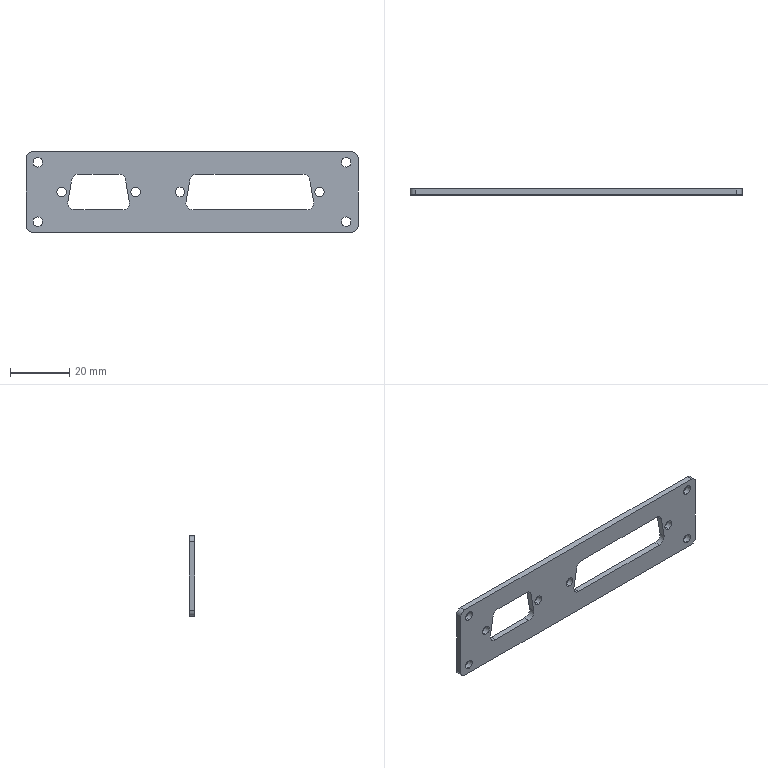Part | SolidWorks | features Cut 1, Extrusion 1, Fillet 1, ICE 1 | 1 solid | 42 faces | box 112 x 2 x 27 mm | volume 4446 mm3 | cylinder 28 | plane 14 | commonest cylinder face diameters 3.2 x16 4.8 x8 4 x4
STEP:
#1=CARTESIAN_POINT('',(43.02,0.,-1.6));
#2=VERTEX_POINT('',#1);
#3=CARTESIAN_POINT('',(43.02,0.,1.6));
#4=VERTEX_POINT('',#3);
#5=CARTESIAN_POINT('',(43.02,0.,0.));
#6=DIRECTION('',(0.,1.,0.));
#7=DIRECTION('',(0.,0.,1.));
#8=AXIS2_PLACEMENT_3D('',#5,#6,#7);
#9=CIRCLE('',#8,1.6);
#10=EDGE_CURVE('',#2,#4,#9,.T.);
#11=ORIENTED_EDGE('',*,*,#10,.F.);
#12=CARTESIAN_POINT('',(43.02,2.,-1.6));
#13=VERTEX_POINT('',#12);
#14=CARTESIAN_POINT('',(43.02,0.,-1.6));
#15=DIRECTION('',(0.,1.,0.));
#16=VECTOR('',#15,1000.);
#17=LINE('',#14,#16);
#18=EDGE_CURVE('',#2,#13,#17,.T.);
#19=ORIENTED_EDGE('',*,*,#18,.T.);
#20=CARTESIAN_POINT('',(43.02,2.,1.6));
#21=VERTEX_POINT('',#20);
#22=CARTESIAN_POINT('',(43.02,2.,0.));
#23=DIRECTION('',(0.,1.,0.));
#24=DIRECTION('',(0.,0.,1.));
#25=AXIS2_PLACEMENT_3D('',#22,#23,#24);
#26=CIRCLE('',#25,1.6);
#27=EDGE_CURVE('',#13,#21,#26,.T.);
#28=ORIENTED_EDGE('',*,*,#27,.T.);
#29=CARTESIAN_POINT('',(43.02,0.,1.6));
#30=DIRECTION('',(0.,1.,0.));
#31=VECTOR('',#30,1000.);
#32=LINE('',#29,#31);
#33=EDGE_CURVE('',#4,#21,#32,.T.);
#34=ORIENTED_EDGE('',*,*,#33,.F.);
#35=EDGE_LOOP('',(#11,#19,#28,#34));
#36=FACE_OUTER_BOUND('',#35,.T.);
#37=CARTESIAN_POINT('',(43.02,0.,0.));
#38=DIRECTION('',(0.,1.,0.));
#39=DIRECTION('',(0.,0.,1.));
#40=AXIS2_PLACEMENT_3D('',#37,#38,#39);
#41=CYLINDRICAL_SURFACE('',#40,1.6);
#42=ADVANCED_FACE('',(#36),#41,.F.);
#43=CARTESIAN_POINT('',(-4.02,0.,-1.6));
#44=VERTEX_POINT('',#43);
#45=CARTESIAN_POINT('',(-4.02,0.,1.6));
#46=VERTEX_POINT('',#45);
#47=CARTESIAN_POINT('',(-4.02,0.,0.));
#48=DIRECTION('',(0.,1.,0.));
#49=DIRECTION('',(0.,0.,1.));
#50=AXIS2_PLACEMENT_3D('',#47,#48,#49);
#51=CIRCLE('',#50,1.6);
#52=EDGE_CURVE('',#44,#46,#51,.T.);
#53=ORIENTED_EDGE('',*,*,#52,.F.);
#54=CARTESIAN_POINT('',(-4.02,2.,-1.6));
#55=VERTEX_POINT('',#54);
#56=CARTESIAN_POINT('',(-4.02,0.,-1.6));
#57=DIRECTION('',(0.,1.,0.));
#58=VECTOR('',#57,1000.);
#59=LINE('',#56,#58);
#60=EDGE_CURVE('',#44,#55,#59,.T.);
#61=ORIENTED_EDGE('',*,*,#60,.T.);
#62=CARTESIAN_POINT('',(-4.02,2.,1.6));
#63=VERTEX_POINT('',#62);
#64=CARTESIAN_POINT('',(-4.02,2.,0.));
#65=DIRECTION('',(0.,1.,0.));
#66=DIRECTION('',(0.,0.,1.));
#67=AXIS2_PLACEMENT_3D('',#64,#65,#66);
#68=CIRCLE('',#67,1.6);
#69=EDGE_CURVE('',#55,#63,#68,.T.);
#70=ORIENTED_EDGE('',*,*,#69,.T.);
#71=CARTESIAN_POINT('',(-4.02,0.,1.6));
#72=DIRECTION('',(0.,1.,0.));
#73=VECTOR('',#72,1000.);
#74=LINE('',#71,#73);
#75=EDGE_CURVE('',#46,#63,#74,.T.);
#76=ORIENTED_EDGE('',*,*,#75,.F.);
#77=EDGE_LOOP('',(#53,#61,#70,#76));
#78=FACE_OUTER_BOUND('',#77,.T.);
#79=CARTESIAN_POINT('',(-4.02,0.,0.));
#80=DIRECTION('',(0.,1.,0.));
#81=DIRECTION('',(0.,0.,1.));
#82=AXIS2_PLACEMENT_3D('',#79,#80,#81);
#83=CYLINDRICAL_SURFACE('',#82,1.6);
#84=ADVANCED_FACE('',(#78),#83,.F.);
#85=CARTESIAN_POINT('',(-19.005,0.,-1.6));
#86=VERTEX_POINT('',#85);
#87=CARTESIAN_POINT('',(-19.005,0.,1.6));
#88=VERTEX_POINT('',#87);
#89=CARTESIAN_POINT('',(-19.005,0.,0.));
#90=DIRECTION('',(0.,1.,0.));
#91=DIRECTION('',(0.,0.,1.));
#92=AXIS2_PLACEMENT_3D('',#89,#90,#91);
#93=CIRCLE('',#92,1.6);
#94=EDGE_CURVE('',#86,#88,#93,.T.);
#95=ORIENTED_EDGE('',*,*,#94,.F.);
#96=CARTESIAN_POINT('',(-19.005,2.,-1.6));
#97=VERTEX_POINT('',#96);
#98=CARTESIAN_POINT('',(-19.005,0.,-1.6));
#99=DIRECTION('',(0.,1.,0.));
#100=VECTOR('',#99,1000.);
#101=LINE('',#98,#100);
#102=EDGE_CURVE('',#86,#97,#101,.T.);
#103=ORIENTED_EDGE('',*,*,#102,.T.);
#104=CARTESIAN_POINT('',(-19.005,2.,1.6));
#105=VERTEX_POINT('',#104);
#106=CARTESIAN_POINT('',(-19.005,2.,0.));
#107=DIRECTION('',(0.,1.,0.));
#108=DIRECTION('',(0.,0.,1.));
#109=AXIS2_PLACEMENT_3D('',#106,#107,#108);
#110=CIRCLE('',#109,1.6);
#111=EDGE_CURVE('',#97,#105,#110,.T.);
#112=ORIENTED_EDGE('',*,*,#111,.T.);
#113=CARTESIAN_POINT('',(-19.005,0.,1.6));
#114=DIRECTION('',(0.,1.,0.));
#115=VECTOR('',#114,1000.);
#116=LINE('',#113,#115);
#117=EDGE_CURVE('',#88,#105,#116,.T.);
#118=ORIENTED_EDGE('',*,*,#117,.F.);
#119=EDGE_LOOP('',(#95,#103,#112,#118));
#120=FACE_OUTER_BOUND('',#119,.T.);
#121=CARTESIAN_POINT('',(-19.005,0.,0.));
#122=DIRECTION('',(0.,1.,0.));
#123=DIRECTION('',(0.,0.,1.));
#124=AXIS2_PLACEMENT_3D('',#121,#122,#123);
#125=CYLINDRICAL_SURFACE('',#124,1.6);
#126=ADVANCED_FACE('',(#120),#125,.F.);
#127=CARTESIAN_POINT('',(-43.995,0.,-1.6));
#128=VERTEX_POINT('',#127);
#129=CARTESIAN_POINT('',(-43.995,0.,1.6));
#130=VERTEX_POINT('',#129);
#131=CARTESIAN_POINT('',(-43.995,0.,0.));
#132=DIRECTION('',(0.,1.,0.));
#133=DIRECTION('',(0.,0.,1.));
#134=AXIS2_PLACEMENT_3D('',#131,#132,#133);
#135=CIRCLE('',#134,1.6);
#136=EDGE_CURVE('',#128,#130,#135,.T.);
#137=ORIENTED_EDGE('',*,*,#136,.F.);
#138=CARTESIAN_POINT('',(-43.995,2.,-1.6));
#139=VERTEX_POINT('',#138);
#140=CARTESIAN_POINT('',(-43.995,0.,-1.6));
#141=DIRECTION('',(0.,1.,0.));
#142=VECTOR('',#141,1000.);
#143=LINE('',#140,#142);
#144=EDGE_CURVE('',#128,#139,#143,.T.);
#145=ORIENTED_EDGE('',*,*,#144,.T.);
#146=CARTESIAN_POINT('',(-43.995,2.,1.6));
#147=VERTEX_POINT('',#146);
#148=CARTESIAN_POINT('',(-43.995,2.,0.));
#149=DIRECTION('',(0.,1.,0.));
#150=DIRECTION('',(0.,0.,1.));
#151=AXIS2_PLACEMENT_3D('',#148,#149,#150);
#152=CIRCLE('',#151,1.6);
#153=EDGE_CURVE('',#139,#147,#152,.T.);
#154=ORIENTED_EDGE('',*,*,#153,.T.);
#155=CARTESIAN_POINT('',(-43.995,0.,1.6));
#156=DIRECTION('',(0.,1.,0.));
#157=VECTOR('',#156,1000.);
#158=LINE('',#155,#157);
#159=EDGE_CURVE('',#130,#147,#158,.T.);
#160=ORIENTED_EDGE('',*,*,#159,.F.);
#161=EDGE_LOOP('',(#137,#145,#154,#160));
#162=FACE_OUTER_BOUND('',#161,.T.);
#163=CARTESIAN_POINT('',(-43.995,0.,0.));
#164=DIRECTION('',(0.,1.,0.));
#165=DIRECTION('',(0.,0.,1.));
#166=AXIS2_PLACEMENT_3D('',#163,#164,#165);
#167=CYLINDRICAL_SURFACE('',#166,1.6);
#168=ADVANCED_FACE('',(#162),#167,.F.);
#169=CARTESIAN_POINT('',(-52.,0.,8.4));
#170=VERTEX_POINT('',#169);
#171=CARTESIAN_POINT('',(-52.,0.,11.6));
#172=VERTEX_POINT('',#171);
#173=CARTESIAN_POINT('',(-52.,0.,10.));
#174=DIRECTION('',(0.,1.,0.));
#175=DIRECTION('',(0.,0.,1.));
#176=AXIS2_PLACEMENT_3D('',#173,#174,#175);
#177=CIRCLE('',#176,1.6);
#178=EDGE_CURVE('',#170,#172,#177,.T.);
#179=ORIENTED_EDGE('',*,*,#178,.F.);
#180=CARTESIAN_POINT('',(-52.,2.,8.4));
#181=VERTEX_POINT('',#180);
#182=CARTESIAN_POINT('',(-52.,0.,8.4));
#183=DIRECTION('',(0.,1.,0.));
#184=VECTOR('',#183,1000.);
#185=LINE('',#182,#184);
#186=EDGE_CURVE('',#170,#181,#185,.T.);
#187=ORIENTED_EDGE('',*,*,#186,.T.);
#188=CARTESIAN_POINT('',(-52.,2.,11.6));
#189=VERTEX_POINT('',#188);
#190=CARTESIAN_POINT('',(-52.,2.,10.));
#191=DIRECTION('',(0.,1.,0.));
#192=DIRECTION('',(0.,0.,1.));
#193=AXIS2_PLACEMENT_3D('',#190,#191,#192);
#194=CIRCLE('',#193,1.6);
#195=EDGE_CURVE('',#181,#189,#194,.T.);
#196=ORIENTED_EDGE('',*,*,#195,.T.);
#197=CARTESIAN_POINT('',(-52.,0.,11.6));
#198=DIRECTION('',(0.,1.,0.));
#199=VECTOR('',#198,1000.);
#200=LINE('',#197,#199);
#201=EDGE_CURVE('',#172,#189,#200,.T.);
#202=ORIENTED_EDGE('',*,*,#201,.F.);
#203=EDGE_LOOP('',(#179,#187,#196,#202));
#204=FACE_OUTER_BOUND('',#203,.T.);
#205=CARTESIAN_POINT('',(-52.,0.,10.));
#206=DIRECTION('',(0.,1.,0.));
#207=DIRECTION('',(0.,0.,1.));
#208=AXIS2_PLACEMENT_3D('',#205,#206,#207);
#209=CYLINDRICAL_SURFACE('',#208,1.6);
#210=ADVANCED_FACE('',(#204),#209,.F.);
#211=CARTESIAN_POINT('',(52.,0.,8.4));
#212=VERTEX_POINT('',#211);
#213=CARTESIAN_POINT('',(52.,0.,11.6));
#214=VERTEX_POINT('',#213);
#215=CARTESIAN_POINT('',(52.,0.,10.));
#216=DIRECTION('',(0.,1.,0.));
#217=DIRECTION('',(0.,0.,1.));
#218=AXIS2_PLACEMENT_3D('',#215,#216,#217);
#219=CIRCLE('',#218,1.6);
#220=EDGE_CURVE('',#212,#214,#219,.T.);
#221=ORIENTED_EDGE('',*,*,#220,.F.);
#222=CARTESIAN_POINT('',(52.,2.,8.4));
#223=VERTEX_POINT('',#222);
#224=CARTESIAN_POINT('',(52.,0.,8.4));
#225=DIRECTION('',(0.,1.,0.));
#226=VECTOR('',#225,1000.);
#227=LINE('',#224,#226);
#228=EDGE_CURVE('',#212,#223,#227,.T.);
#229=ORIENTED_EDGE('',*,*,#228,.T.);
#230=CARTESIAN_POINT('',(52.,2.,11.6));
#231=VERTEX_POINT('',#230);
#232=CARTESIAN_POINT('',(52.,2.,10.));
#233=DIRECTION('',(0.,1.,0.));
#234=DIRECTION('',(0.,0.,1.));
#235=AXIS2_PLACEMENT_3D('',#232,#233,#234);
#236=CIRCLE('',#235,1.6);
#237=EDGE_CURVE('',#223,#231,#236,.T.);
#238=ORIENTED_EDGE('',*,*,#237,.T.);
#239=CARTESIAN_POINT('',(52.,0.,11.6));
#240=DIRECTION('',(0.,1.,0.));
#241=VECTOR('',#240,1000.);
#242=LINE('',#239,#241);
#243=EDGE_CURVE('',#214,#231,#242,.T.);
#244=ORIENTED_EDGE('',*,*,#243,.F.);
#245=EDGE_LOOP('',(#221,#229,#238,#244));
#246=FACE_OUTER_BOUND('',#245,.T.);
#247=CARTESIAN_POINT('',(52.,0.,10.));
#248=DIRECTION('',(0.,1.,0.));
#249=DIRECTION('',(0.,0.,1.));
#250=AXIS2_PLACEMENT_3D('',#247,#248,#249);
#251=CYLINDRICAL_SURFACE('',#250,1.6);
#252=ADVANCED_FACE('',(#246),#251,.F.);
#253=CARTESIAN_POINT('',(52.,0.,-11.6));
#254=VERTEX_POINT('',#253);
#255=CARTESIAN_POINT('',(52.,0.,-8.4));
#256=VERTEX_POINT('',#255);
#257=CARTESIAN_POINT('',(52.,0.,-10.));
#258=DIRECTION('',(0.,1.,0.));
#259=DIRECTION('',(0.,0.,1.));
#260=AXIS2_PLACEMENT_3D('',#257,#258,#259);
#261=CIRCLE('',#260,1.6);
#262=EDGE_CURVE('',#254,#256,#261,.T.);
#263=ORIENTED_EDGE('',*,*,#262,.F.);
#264=CARTESIAN_POINT('',(52.,2.,-11.6));
#265=VERTEX_POINT('',#264);
#266=CARTESIAN_POINT('',(52.,0.,-11.6));
#267=DIRECTION('',(0.,1.,0.));
#268=VECTOR('',#267,1000.);
#269=LINE('',#266,#268);
#270=EDGE_CURVE('',#254,#265,#269,.T.);
#271=ORIENTED_EDGE('',*,*,#270,.T.);
#272=CARTESIAN_POINT('',(52.,2.,-8.4));
#273=VERTEX_POINT('',#272);
#274=CARTESIAN_POINT('',(52.,2.,-10.));
#275=DIRECTION('',(0.,1.,0.));
#276=DIRECTION('',(0.,0.,1.));
#277=AXIS2_PLACEMENT_3D('',#274,#275,#276);
#278=CIRCLE('',#277,1.6);
#279=EDGE_CURVE('',#265,#273,#278,.T.);
#280=ORIENTED_EDGE('',*,*,#279,.T.);
#281=CARTESIAN_POINT('',(52.,0.,-8.4));
#282=DIRECTION('',(0.,1.,0.));
#283=VECTOR('',#282,1000.);
#284=LINE('',#281,#283);
#285=EDGE_CURVE('',#256,#273,#284,.T.);
#286=ORIENTED_EDGE('',*,*,#285,.F.);
#287=EDGE_LOOP('',(#263,#271,#280,#286));
#288=FACE_OUTER_BOUND('',#287,.T.);
#289=CARTESIAN_POINT('',(52.,0.,-10.));
#290=DIRECTION('',(0.,1.,0.));
#291=DIRECTION('',(0.,0.,1.));
#292=AXIS2_PLACEMENT_3D('',#289,#290,#291);
#293=CYLINDRICAL_SURFACE('',#292,1.6);
#294=ADVANCED_FACE('',(#288),#293,.F.);
#295=CARTESIAN_POINT('',(-52.,0.,-11.6));
#296=VERTEX_POINT('',#295);
#297=CARTESIAN_POINT('',(-52.,0.,-8.4));
#298=VERTEX_POINT('',#297);
#299=CARTESIAN_POINT('',(-52.,0.,-10.));
#300=DIRECTION('',(0.,1.,0.));
#301=DIRECTION('',(0.,0.,1.));
#302=AXIS2_PLACEMENT_3D('',#299,#300,#301);
#303=CIRCLE('',#302,1.6);
#304=EDGE_CURVE('',#296,#298,#303,.T.);
#305=ORIENTED_EDGE('',*,*,#304,.F.);
#306=CARTESIAN_POINT('',(-52.,2.,-11.6));
#307=VERTEX_POINT('',#306);
#308=CARTESIAN_POINT('',(-52.,0.,-11.6));
#309=DIRECTION('',(0.,1.,0.));
#310=VECTOR('',#309,1000.);
#311=LINE('',#308,#310);
#312=EDGE_CURVE('',#296,#307,#311,.T.);
#313=ORIENTED_EDGE('',*,*,#312,.T.);
#314=CARTESIAN_POINT('',(-52.,2.,-8.4));
#315=VERTEX_POINT('',#314);
#316=CARTESIAN_POINT('',(-52.,2.,-10.));
#317=DIRECTION('',(0.,1.,0.));
#318=DIRECTION('',(0.,0.,1.));
#319=AXIS2_PLACEMENT_3D('',#316,#317,#318);
#320=CIRCLE('',#319,1.6);
#321=EDGE_CURVE('',#307,#315,#320,.T.);
#322=ORIENTED_EDGE('',*,*,#321,.T.);
#323=CARTESIAN_POINT('',(-52.,0.,-8.4));
#324=DIRECTION('',(0.,1.,0.));
#325=VECTOR('',#324,1000.);
#326=LINE('',#323,#325);
#327=EDGE_CURVE('',#298,#315,#326,.T.);
#328=ORIENTED_EDGE('',*,*,#327,.F.);
#329=EDGE_LOOP('',(#305,#313,#322,#328));
#330=FACE_OUTER_BOUND('',#329,.T.);
#331=CARTESIAN_POINT('',(-52.,0.,-10.));
#332=DIRECTION('',(0.,1.,0.));
#333=DIRECTION('',(0.,0.,1.));
#334=AXIS2_PLACEMENT_3D('',#331,#332,#333);
#335=CYLINDRICAL_SURFACE('',#334,1.6);
#336=ADVANCED_FACE('',(#330),#335,.F.);
#337=CARTESIAN_POINT('',(43.02,2.,0.));
#338=DIRECTION('',(0.,1.,0.));
#339=DIRECTION('',(0.,0.,1.));
#340=AXIS2_PLACEMENT_3D('',#337,#338,#339);
#341=CIRCLE('',#340,1.6);
#342=EDGE_CURVE('',#21,#13,#341,.T.);
#343=ORIENTED_EDGE('',*,*,#342,.F.);
#344=ORIENTED_EDGE('',*,*,#27,.F.);
#345=EDGE_LOOP('',(#343,#344));
#346=FACE_BOUND('',#345,.T.);
#347=CARTESIAN_POINT('',(-39.5,2.,-6.05));
#348=VERTEX_POINT('',#347);
#349=CARTESIAN_POINT('',(-23.5,2.,-6.05));
#350=VERTEX_POINT('',#349);
#351=CARTESIAN_POINT('',(0.,2.,-6.05));
#352=DIRECTION('',(1.,0.,0.));
#353=VECTOR('',#352,1000.);
#354=LINE('',#351,#353);
#355=EDGE_CURVE('',#348,#350,#354,.T.);
#356=ORIENTED_EDGE('',*,*,#355,.T.);
#357=CARTESIAN_POINT('',(-21.136,2.,-3.233));
#358=VERTEX_POINT('',#357);
#359=CARTESIAN_POINT('',(-23.5,2.,-3.65));
#360=DIRECTION('',(0.,-1.,0.));
#361=DIRECTION('',(0.,0.,1.));
#362=AXIS2_PLACEMENT_3D('',#359,#360,#361);
#363=CIRCLE('',#362,2.4);
#364=EDGE_CURVE('',#350,#358,#363,.T.);
#365=ORIENTED_EDGE('',*,*,#364,.T.);
#366=CARTESIAN_POINT('',(-22.424,2.,4.067));
#367=VERTEX_POINT('',#366);
#368=CARTESIAN_POINT('',(-21.052,2.,-3.712));
#369=DIRECTION('',(-0.1736,0.,0.9848));
#370=VECTOR('',#369,1000.);
#371=LINE('',#368,#370);
#372=EDGE_CURVE('',#358,#367,#371,.T.);
#373=ORIENTED_EDGE('',*,*,#372,.T.);
#374=CARTESIAN_POINT('',(-24.787,2.,6.05));
#375=VERTEX_POINT('',#374);
#376=CARTESIAN_POINT('',(-24.787,2.,3.65));
#377=DIRECTION('',(0.,-1.,0.));
#378=DIRECTION('',(0.,0.,1.));
#379=AXIS2_PLACEMENT_3D('',#376,#377,#378);
#380=CIRCLE('',#379,2.4);
#381=EDGE_CURVE('',#367,#375,#380,.T.);
#382=ORIENTED_EDGE('',*,*,#381,.T.);
#383=CARTESIAN_POINT('',(-38.213,2.,6.05));
#384=VERTEX_POINT('',#383);
#385=CARTESIAN_POINT('',(0.,2.,6.05));
#386=DIRECTION('',(-1.,0.,0.));
#387=VECTOR('',#386,1000.);
#388=LINE('',#385,#387);
#389=EDGE_CURVE('',#375,#384,#388,.T.);
#390=ORIENTED_EDGE('',*,*,#389,.T.);
#391=CARTESIAN_POINT('',(-40.576,2.,4.067));
#392=VERTEX_POINT('',#391);
#393=CARTESIAN_POINT('',(-38.213,2.,3.65));
#394=DIRECTION('',(0.,-1.,0.));
#395=DIRECTION('',(0.,0.,1.));
#396=AXIS2_PLACEMENT_3D('',#393,#394,#395);
#397=CIRCLE('',#396,2.4);
#398=EDGE_CURVE('',#384,#392,#397,.T.);
#399=ORIENTED_EDGE('',*,*,#398,.T.);
#400=CARTESIAN_POINT('',(-41.864,2.,-3.233));
#401=VERTEX_POINT('',#400);
#402=CARTESIAN_POINT('',(-40.048,2.,7.062));
#403=DIRECTION('',(-0.1736,0.,-0.9848));
#404=VECTOR('',#403,1000.);
#405=LINE('',#402,#404);
#406=EDGE_CURVE('',#392,#401,#405,.T.);
#407=ORIENTED_EDGE('',*,*,#406,.T.);
#408=CARTESIAN_POINT('',(-39.5,2.,-3.65));
#409=DIRECTION('',(0.,1.,0.));
#410=DIRECTION('',(0.,0.,1.));
#411=AXIS2_PLACEMENT_3D('',#408,#409,#410);
#412=CIRCLE('',#411,2.4);
#413=EDGE_CURVE('',#348,#401,#412,.T.);
#414=ORIENTED_EDGE('',*,*,#413,.F.);
#415=EDGE_LOOP('',(#356,#365,#373,#382,#390,#399,#407,#414));
#416=FACE_BOUND('',#415,.T.);
#417=CARTESIAN_POINT('',(-52.,2.,10.));
#418=DIRECTION('',(0.,1.,0.));
#419=DIRECTION('',(0.,0.,1.));
#420=AXIS2_PLACEMENT_3D('',#417,#418,#419);
#421=CIRCLE('',#420,1.6);
#422=EDGE_CURVE('',#189,#181,#421,.T.);
#423=ORIENTED_EDGE('',*,*,#422,.F.);
#424=ORIENTED_EDGE('',*,*,#195,.F.);
#425=EDGE_LOOP('',(#423,#424));
#426=FACE_BOUND('',#425,.T.);
#427=CARTESIAN_POINT('',(52.,2.,10.));
#428=DIRECTION('',(0.,1.,0.));
#429=DIRECTION('',(0.,0.,1.));
#430=AXIS2_PLACEMENT_3D('',#427,#428,#429);
#431=CIRCLE('',#430,1.6);
#432=EDGE_CURVE('',#231,#223,#431,.T.);
#433=ORIENTED_EDGE('',*,*,#432,.F.);
#434=ORIENTED_EDGE('',*,*,#237,.F.);
#435=EDGE_LOOP('',(#433,#434));
#436=FACE_BOUND('',#435,.T.);
#437=CARTESIAN_POINT('',(52.,2.,-10.));
#438=DIRECTION('',(0.,1.,0.));
#439=DIRECTION('',(0.,0.,1.));
#440=AXIS2_PLACEMENT_3D('',#437,#438,#439);
#441=CIRCLE('',#440,1.6);
#442=EDGE_CURVE('',#273,#265,#441,.T.);
#443=ORIENTED_EDGE('',*,*,#442,.F.);
#444=ORIENTED_EDGE('',*,*,#279,.F.);
#445=EDGE_LOOP('',(#443,#444));
#446=FACE_BOUND('',#445,.T.);
#447=CARTESIAN_POINT('',(-52.,2.,-10.));
#448=DIRECTION('',(0.,1.,0.));
#449=DIRECTION('',(0.,0.,1.));
#450=AXIS2_PLACEMENT_3D('',#447,#448,#449);
#451=CIRCLE('',#450,1.6);
#452=EDGE_CURVE('',#315,#307,#451,.T.);
#453=ORIENTED_EDGE('',*,*,#452,.F.);
#454=ORIENTED_EDGE('',*,*,#321,.F.);
#455=EDGE_LOOP('',(#453,#454));
#456=FACE_BOUND('',#455,.T.);
#457=CARTESIAN_POINT('',(56.,2.,11.5));
#458=VERTEX_POINT('',#457);
#459=CARTESIAN_POINT('',(56.,2.,-11.5));
#460=VERTEX_POINT('',#459);
#461=CARTESIAN_POINT('',(56.,2.,13.5));
#462=DIRECTION('',(0.,0.,-1.));
#463=VECTOR('',#462,1000.);
#464=LINE('',#461,#463);
#465=EDGE_CURVE('',#458,#460,#464,.T.);
#466=ORIENTED_EDGE('',*,*,#465,.T.);
#467=CARTESIAN_POINT('',(54.,2.,-13.5));
#468=VERTEX_POINT('',#467);
#469=CARTESIAN_POINT('',(54.,2.,-11.5));
#470=DIRECTION('',(0.,1.,0.));
#471=DIRECTION('',(0.,0.,-1.));
#472=AXIS2_PLACEMENT_3D('',#469,#470,#471);
#473=CIRCLE('',#472,2.);
#474=EDGE_CURVE('',#460,#468,#473,.T.);
#475=ORIENTED_EDGE('',*,*,#474,.T.);
#476=CARTESIAN_POINT('',(-54.,2.,-13.5));
#477=VERTEX_POINT('',#476);
#478=CARTESIAN_POINT('',(-56.,2.,-13.5));
#479=DIRECTION('',(-1.,0.,0.));
#480=VECTOR('',#479,1000.);
#481=LINE('',#478,#480);
#482=EDGE_CURVE('',#468,#477,#481,.T.);
#483=ORIENTED_EDGE('',*,*,#482,.T.);
#484=CARTESIAN_POINT('',(-56.,2.,-11.5));
#485=VERTEX_POINT('',#484);
#486=CARTESIAN_POINT('',(-54.,2.,-11.5));
#487=DIRECTION('',(0.,1.,0.));
#488=DIRECTION('',(0.,0.,-1.));
#489=AXIS2_PLACEMENT_3D('',#486,#487,#488);
#490=CIRCLE('',#489,2.);
#491=EDGE_CURVE('',#477,#485,#490,.T.);
#492=ORIENTED_EDGE('',*,*,#491,.T.);
#493=CARTESIAN_POINT('',(-56.,2.,11.5));
#494=VERTEX_POINT('',#493);
#495=CARTESIAN_POINT('',(-56.,2.,13.5));
#496=DIRECTION('',(0.,0.,1.));
#497=VECTOR('',#496,1000.);
#498=LINE('',#495,#497);
#499=EDGE_CURVE('',#485,#494,#498,.T.);
#500=ORIENTED_EDGE('',*,*,#499,.T.);
#501=CARTESIAN_POINT('',(-54.,2.,13.5));
#502=VERTEX_POINT('',#501);
#503=CARTESIAN_POINT('',(-54.,2.,11.5));
#504=DIRECTION('',(0.,1.,0.));
#505=DIRECTION('',(0.,0.,-1.));
#506=AXIS2_PLACEMENT_3D('',#503,#504,#505);
#507=CIRCLE('',#506,2.);
#508=EDGE_CURVE('',#494,#502,#507,.T.);
#509=ORIENTED_EDGE('',*,*,#508,.T.);
#510=CARTESIAN_POINT('',(54.,2.,13.5));
#511=VERTEX_POINT('',#510);
#512=CARTESIAN_POINT('',(-56.,2.,13.5));
#513=DIRECTION('',(1.,0.,0.));
#514=VECTOR('',#513,1000.);
#515=LINE('',#512,#514);
#516=EDGE_CURVE('',#502,#511,#515,.T.);
#517=ORIENTED_EDGE('',*,*,#516,.T.);
#518=CARTESIAN_POINT('',(54.,2.,11.5));
#519=DIRECTION('',(0.,1.,0.));
#520=DIRECTION('',(0.,0.,-1.));
#521=AXIS2_PLACEMENT_3D('',#518,#519,#520);
#522=CIRCLE('',#521,2.);
#523=EDGE_CURVE('',#511,#458,#522,.T.);
#524=ORIENTED_EDGE('',*,*,#523,.T.);
#525=EDGE_LOOP('',(#466,#475,#483,#492,#500,#509,#517,#524));
#526=FACE_OUTER_BOUND('',#525,.T.);
#527=CARTESIAN_POINT('',(-43.995,2.,0.));
#528=DIRECTION('',(0.,1.,0.));
#529=DIRECTION('',(0.,0.,1.));
#530=AXIS2_PLACEMENT_3D('',#527,#528,#529);
#531=CIRCLE('',#530,1.6);
#532=EDGE_CURVE('',#147,#139,#531,.T.);
#533=ORIENTED_EDGE('',*,*,#532,.F.);
#534=ORIENTED_EDGE('',*,*,#153,.F.);
#535=EDGE_LOOP('',(#533,#534));
#536=FACE_BOUND('',#535,.T.);
#537=CARTESIAN_POINT('',(-19.005,2.,0.));
#538=DIRECTION('',(0.,1.,0.));
#539=DIRECTION('',(0.,0.,1.));
#540=AXIS2_PLACEMENT_3D('',#537,#538,#539);
#541=CIRCLE('',#540,1.6);
#542=EDGE_CURVE('',#105,#97,#541,.T.);
#543=ORIENTED_EDGE('',*,*,#542,.F.);
#544=ORIENTED_EDGE('',*,*,#111,.F.);
#545=EDGE_LOOP('',(#543,#544));
#546=FACE_BOUND('',#545,.T.);
#547=CARTESIAN_POINT('',(-4.02,2.,0.));
#548=DIRECTION('',(0.,1.,0.));
#549=DIRECTION('',(0.,0.,1.));
#550=AXIS2_PLACEMENT_3D('',#547,#548,#549);
#551=CIRCLE('',#550,1.6);
#552=EDGE_CURVE('',#63,#55,#551,.T.);
#553=ORIENTED_EDGE('',*,*,#552,.F.);
#554=ORIENTED_EDGE('',*,*,#69,.F.);
#555=EDGE_LOOP('',(#553,#554));
#556=FACE_BOUND('',#555,.T.);
#557=CARTESIAN_POINT('',(39.726,2.,4.067));
#558=VERTEX_POINT('',#557);
#559=CARTESIAN_POINT('',(37.363,2.,6.05));
#560=VERTEX_POINT('',#559);
#561=CARTESIAN_POINT('',(37.363,2.,3.65));
#562=DIRECTION('',(0.,-1.,0.));
#563=DIRECTION('',(0.,0.,1.));
#564=AXIS2_PLACEMENT_3D('',#561,#562,#563);
#565=CIRCLE('',#564,2.4);
#566=EDGE_CURVE('',#558,#560,#565,.T.);
#567=ORIENTED_EDGE('',*,*,#566,.T.);
#568=CARTESIAN_POINT('',(1.637,2.,6.05));
#569=VERTEX_POINT('',#568);
#570=CARTESIAN_POINT('',(0.,2.,6.05));
#571=DIRECTION('',(-1.,0.,0.));
#572=VECTOR('',#571,1000.);
#573=LINE('',#570,#572);
#574=EDGE_CURVE('',#560,#569,#573,.T.);
#575=ORIENTED_EDGE('',*,*,#574,.T.);
#576=CARTESIAN_POINT('',(-0.7264,2.,4.067));
#577=VERTEX_POINT('',#576);
#578=CARTESIAN_POINT('',(1.637,2.,3.65));
#579=DIRECTION('',(0.,-1.,0.));
#580=DIRECTION('',(0.,0.,1.));
#581=AXIS2_PLACEMENT_3D('',#578,#579,#580);
#582=CIRCLE('',#581,2.4);
#583=EDGE_CURVE('',#569,#577,#582,.T.);
#584=ORIENTED_EDGE('',*,*,#583,.T.);
#585=CARTESIAN_POINT('',(-2.014,2.,-3.233));
#586=VERTEX_POINT('',#585);
#587=CARTESIAN_POINT('',(-1.4,2.,0.2468));
#588=DIRECTION('',(-0.1736,0.,-0.9848));
#589=VECTOR('',#588,1000.);
#590=LINE('',#587,#589);
#591=EDGE_CURVE('',#577,#586,#590,.T.);
#592=ORIENTED_EDGE('',*,*,#591,.T.);
#593=CARTESIAN_POINT('',(0.35,2.,-6.05));
#594=VERTEX_POINT('',#593);
#595=CARTESIAN_POINT('',(0.35,2.,-3.65));
#596=DIRECTION('',(0.,1.,0.));
#597=DIRECTION('',(0.,0.,1.));
#598=AXIS2_PLACEMENT_3D('',#595,#596,#597);
#599=CIRCLE('',#598,2.4);
#600=EDGE_CURVE('',#594,#586,#599,.T.);
#601=ORIENTED_EDGE('',*,*,#600,.F.);
#602=CARTESIAN_POINT('',(38.65,2.,-6.05));
#603=VERTEX_POINT('',#602);
#604=CARTESIAN_POINT('',(0.,2.,-6.05));
#605=DIRECTION('',(1.,0.,0.));
#606=VECTOR('',#605,1000.);
#607=LINE('',#604,#606);
#608=EDGE_CURVE('',#594,#603,#607,.T.);
#609=ORIENTED_EDGE('',*,*,#608,.T.);
#610=CARTESIAN_POINT('',(41.014,2.,-3.233));
#611=VERTEX_POINT('',#610);
#612=CARTESIAN_POINT('',(38.65,2.,-3.65));
#613=DIRECTION('',(0.,-1.,0.));
#614=DIRECTION('',(0.,0.,1.));
#615=AXIS2_PLACEMENT_3D('',#612,#613,#614);
#616=CIRCLE('',#615,2.4);
#617=EDGE_CURVE('',#603,#611,#616,.T.);
#618=ORIENTED_EDGE('',*,*,#617,.T.);
#619=CARTESIAN_POINT('',(39.224,2.,6.916));
#620=DIRECTION('',(-0.1736,0.,0.9848));
#621=VECTOR('',#620,1000.);
#622=LINE('',#619,#621);
#623=EDGE_CURVE('',#611,#558,#622,.T.);
#624=ORIENTED_EDGE('',*,*,#623,.T.);
#625=EDGE_LOOP('',(#567,#575,#584,#592,#601,#609,#618,#624));
#626=FACE_BOUND('',#625,.T.);
#627=CARTESIAN_POINT('',(0.,2.,0.));
#628=DIRECTION('',(0.,-1.,0.));
#629=DIRECTION('',(0.,0.,-1.));
#630=AXIS2_PLACEMENT_3D('',#627,#628,#629);
#631=PLANE('',#630);
#632=ADVANCED_FACE('',(#346,#416,#426,#436,#446,#456,#526,#536,#546,#556,#626),#631,.F.);
#633=CARTESIAN_POINT('',(43.02,0.,0.));
#634=DIRECTION('',(0.,1.,0.));
#635=DIRECTION('',(0.,0.,1.));
#636=AXIS2_PLACEMENT_3D('',#633,#634,#635);
#637=CIRCLE('',#636,1.6);
#638=EDGE_CURVE('',#4,#2,#637,.T.);
#639=ORIENTED_EDGE('',*,*,#638,.T.);
#640=ORIENTED_EDGE('',*,*,#10,.T.);
#641=EDGE_LOOP('',(#639,#640));
#642=FACE_BOUND('',#641,.T.);
#643=CARTESIAN_POINT('',(-4.02,0.,0.));
#644=DIRECTION('',(0.,1.,0.));
#645=DIRECTION('',(0.,0.,1.));
#646=AXIS2_PLACEMENT_3D('',#643,#644,#645);
#647=CIRCLE('',#646,1.6);
#648=EDGE_CURVE('',#46,#44,#647,.T.);
#649=ORIENTED_EDGE('',*,*,#648,.T.);
#650=ORIENTED_EDGE('',*,*,#52,.T.);
#651=EDGE_LOOP('',(#649,#650));
#652=FACE_BOUND('',#651,.T.);
#653=CARTESIAN_POINT('',(-19.005,0.,0.));
#654=DIRECTION('',(0.,1.,0.));
#655=DIRECTION('',(0.,0.,1.));
#656=AXIS2_PLACEMENT_3D('',#653,#654,#655);
#657=CIRCLE('',#656,1.6);
#658=EDGE_CURVE('',#88,#86,#657,.T.);
#659=ORIENTED_EDGE('',*,*,#658,.T.);
#660=ORIENTED_EDGE('',*,*,#94,.T.);
#661=EDGE_LOOP('',(#659,#660));
#662=FACE_BOUND('',#661,.T.);
#663=CARTESIAN_POINT('',(-43.995,0.,0.));
#664=DIRECTION('',(0.,1.,0.));
#665=DIRECTION('',(0.,0.,1.));
#666=AXIS2_PLACEMENT_3D('',#663,#664,#665);
#667=CIRCLE('',#666,1.6);
#668=EDGE_CURVE('',#130,#128,#667,.T.);
#669=ORIENTED_EDGE('',*,*,#668,.T.);
#670=ORIENTED_EDGE('',*,*,#136,.T.);
#671=EDGE_LOOP('',(#669,#670));
#672=FACE_BOUND('',#671,.T.);
#673=CARTESIAN_POINT('',(-52.,0.,10.));
#674=DIRECTION('',(0.,1.,0.));
#675=DIRECTION('',(0.,0.,1.));
#676=AXIS2_PLACEMENT_3D('',#673,#674,#675);
#677=CIRCLE('',#676,1.6);
#678=EDGE_CURVE('',#172,#170,#677,.T.);
#679=ORIENTED_EDGE('',*,*,#678,.T.);
#680=ORIENTED_EDGE('',*,*,#178,.T.);
#681=EDGE_LOOP('',(#679,#680));
#682=FACE_BOUND('',#681,.T.);
#683=CARTESIAN_POINT('',(52.,0.,10.));
#684=DIRECTION('',(0.,1.,0.));
#685=DIRECTION('',(0.,0.,1.));
#686=AXIS2_PLACEMENT_3D('',#683,#684,#685);
#687=CIRCLE('',#686,1.6);
#688=EDGE_CURVE('',#214,#212,#687,.T.);
#689=ORIENTED_EDGE('',*,*,#688,.T.);
#690=ORIENTED_EDGE('',*,*,#220,.T.);
#691=EDGE_LOOP('',(#689,#690));
#692=FACE_BOUND('',#691,.T.);
#693=CARTESIAN_POINT('',(52.,0.,-10.));
#694=DIRECTION('',(0.,1.,0.));
#695=DIRECTION('',(0.,0.,1.));
#696=AXIS2_PLACEMENT_3D('',#693,#694,#695);
#697=CIRCLE('',#696,1.6);
#698=EDGE_CURVE('',#256,#254,#697,.T.);
#699=ORIENTED_EDGE('',*,*,#698,.T.);
#700=ORIENTED_EDGE('',*,*,#262,.T.);
#701=EDGE_LOOP('',(#699,#700));
#702=FACE_BOUND('',#701,.T.);
#703=CARTESIAN_POINT('',(-52.,0.,-10.));
#704=DIRECTION('',(0.,1.,0.));
#705=DIRECTION('',(0.,0.,1.));
#706=AXIS2_PLACEMENT_3D('',#703,#704,#705);
#707=CIRCLE('',#706,1.6);
#708=EDGE_CURVE('',#298,#296,#707,.T.);
#709=ORIENTED_EDGE('',*,*,#708,.T.);
#710=ORIENTED_EDGE('',*,*,#304,.T.);
#711=EDGE_LOOP('',(#709,#710));
#712=FACE_BOUND('',#711,.T.);
#713=CARTESIAN_POINT('',(54.,0.,-13.5));
#714=VERTEX_POINT('',#713);
#715=CARTESIAN_POINT('',(-54.,0.,-13.5));
#716=VERTEX_POINT('',#715);
#717=CARTESIAN_POINT('',(-56.,0.,-13.5));
#718=DIRECTION('',(-1.,0.,0.));
#719=VECTOR('',#718,1000.);
#720=LINE('',#717,#719);
#721=EDGE_CURVE('',#714,#716,#720,.T.);
#722=ORIENTED_EDGE('',*,*,#721,.F.);
#723=CARTESIAN_POINT('',(56.,0.,-11.5));
#724=VERTEX_POINT('',#723);
#725=CARTESIAN_POINT('',(54.,0.,-11.5));
#726=DIRECTION('',(0.,-1.,0.));
#727=DIRECTION('',(0.,0.,-1.));
#728=AXIS2_PLACEMENT_3D('',#725,#726,#727);
#729=CIRCLE('',#728,2.);
#730=EDGE_CURVE('',#714,#724,#729,.T.);
#731=ORIENTED_EDGE('',*,*,#730,.T.);
#732=CARTESIAN_POINT('',(56.,0.,11.5));
#733=VERTEX_POINT('',#732);
#734=CARTESIAN_POINT('',(56.,0.,13.5));
#735=DIRECTION('',(0.,0.,-1.));
#736=VECTOR('',#735,1000.);
#737=LINE('',#734,#736);
#738=EDGE_CURVE('',#733,#724,#737,.T.);
#739=ORIENTED_EDGE('',*,*,#738,.F.);
#740=CARTESIAN_POINT('',(54.,0.,13.5));
#741=VERTEX_POINT('',#740);
#742=CARTESIAN_POINT('',(54.,0.,11.5));
#743=DIRECTION('',(0.,-1.,0.));
#744=DIRECTION('',(0.,0.,-1.));
#745=AXIS2_PLACEMENT_3D('',#742,#743,#744);
#746=CIRCLE('',#745,2.);
#747=EDGE_CURVE('',#733,#741,#746,.T.);
#748=ORIENTED_EDGE('',*,*,#747,.T.);
#749=CARTESIAN_POINT('',(-54.,0.,13.5));
#750=VERTEX_POINT('',#749);
#751=CARTESIAN_POINT('',(-56.,0.,13.5));
#752=DIRECTION('',(1.,0.,0.));
#753=VECTOR('',#752,1000.);
#754=LINE('',#751,#753);
#755=EDGE_CURVE('',#750,#741,#754,.T.);
#756=ORIENTED_EDGE('',*,*,#755,.F.);
#757=CARTESIAN_POINT('',(-56.,0.,11.5));
#758=VERTEX_POINT('',#757);
#759=CARTESIAN_POINT('',(-54.,0.,11.5));
#760=DIRECTION('',(0.,-1.,0.));
#761=DIRECTION('',(0.,0.,-1.));
#762=AXIS2_PLACEMENT_3D('',#759,#760,#761);
#763=CIRCLE('',#762,2.);
#764=EDGE_CURVE('',#750,#758,#763,.T.);
#765=ORIENTED_EDGE('',*,*,#764,.T.);
#766=CARTESIAN_POINT('',(-56.,0.,-11.5));
#767=VERTEX_POINT('',#766);
#768=CARTESIAN_POINT('',(-56.,0.,13.5));
#769=DIRECTION('',(0.,0.,1.));
#770=VECTOR('',#769,1000.);
#771=LINE('',#768,#770);
#772=EDGE_CURVE('',#767,#758,#771,.T.);
#773=ORIENTED_EDGE('',*,*,#772,.F.);
#774=CARTESIAN_POINT('',(-54.,0.,-11.5));
#775=DIRECTION('',(0.,-1.,0.));
#776=DIRECTION('',(0.,0.,-1.));
#777=AXIS2_PLACEMENT_3D('',#774,#775,#776);
#778=CIRCLE('',#777,2.);
#779=EDGE_CURVE('',#767,#716,#778,.T.);
#780=ORIENTED_EDGE('',*,*,#779,.T.);
#781=EDGE_LOOP('',(#722,#731,#739,#748,#756,#765,#773,#780));
#782=FACE_OUTER_BOUND('',#781,.T.);
#783=CARTESIAN_POINT('',(-23.5,0.,-6.05));
#784=VERTEX_POINT('',#783);
#785=CARTESIAN_POINT('',(-21.136,0.,-3.233));
#786=VERTEX_POINT('',#785);
#787=CARTESIAN_POINT('',(-23.5,0.,-3.65));
#788=DIRECTION('',(0.,-1.,0.));
#789=DIRECTION('',(0.,0.,1.));
#790=AXIS2_PLACEMENT_3D('',#787,#788,#789);
#791=CIRCLE('',#790,2.4);
#792=EDGE_CURVE('',#784,#786,#791,.T.);
#793=ORIENTED_EDGE('',*,*,#792,.F.);
#794=CARTESIAN_POINT('',(-39.5,0.,-6.05));
#795=VERTEX_POINT('',#794);
#796=CARTESIAN_POINT('',(0.,0.,-6.05));
#797=DIRECTION('',(1.,0.,0.));
#798=VECTOR('',#797,1000.);
#799=LINE('',#796,#798);
#800=EDGE_CURVE('',#795,#784,#799,.T.);
#801=ORIENTED_EDGE('',*,*,#800,.F.);
#802=CARTESIAN_POINT('',(-41.864,0.,-3.233));
#803=VERTEX_POINT('',#802);
#804=CARTESIAN_POINT('',(-39.5,0.,-3.65));
#805=DIRECTION('',(0.,1.,0.));
#806=DIRECTION('',(0.,0.,1.));
#807=AXIS2_PLACEMENT_3D('',#804,#805,#806);
#808=CIRCLE('',#807,2.4);
#809=EDGE_CURVE('',#795,#803,#808,.T.);
#810=ORIENTED_EDGE('',*,*,#809,.T.);
#811=CARTESIAN_POINT('',(-40.576,0.,4.067));
#812=VERTEX_POINT('',#811);
#813=CARTESIAN_POINT('',(-40.048,0.,7.062));
#814=DIRECTION('',(-0.1736,0.,-0.9848));
#815=VECTOR('',#814,1000.);
#816=LINE('',#813,#815);
#817=EDGE_CURVE('',#812,#803,#816,.T.);
#818=ORIENTED_EDGE('',*,*,#817,.F.);
#819=CARTESIAN_POINT('',(-38.213,0.,6.05));
#820=VERTEX_POINT('',#819);
#821=CARTESIAN_POINT('',(-38.213,0.,3.65));
#822=DIRECTION('',(0.,-1.,0.));
#823=DIRECTION('',(0.,0.,1.));
#824=AXIS2_PLACEMENT_3D('',#821,#822,#823);
#825=CIRCLE('',#824,2.4);
#826=EDGE_CURVE('',#820,#812,#825,.T.);
#827=ORIENTED_EDGE('',*,*,#826,.F.);
#828=CARTESIAN_POINT('',(-24.787,0.,6.05));
#829=VERTEX_POINT('',#828);
#830=CARTESIAN_POINT('',(0.,0.,6.05));
#831=DIRECTION('',(-1.,0.,0.));
#832=VECTOR('',#831,1000.);
#833=LINE('',#830,#832);
#834=EDGE_CURVE('',#829,#820,#833,.T.);
#835=ORIENTED_EDGE('',*,*,#834,.F.);
#836=CARTESIAN_POINT('',(-22.424,0.,4.067));
#837=VERTEX_POINT('',#836);
#838=CARTESIAN_POINT('',(-24.787,0.,3.65));
#839=DIRECTION('',(0.,-1.,0.));
#840=DIRECTION('',(0.,0.,1.));
#841=AXIS2_PLACEMENT_3D('',#838,#839,#840);
#842=CIRCLE('',#841,2.4);
#843=EDGE_CURVE('',#837,#829,#842,.T.);
#844=ORIENTED_EDGE('',*,*,#843,.F.);
#845=CARTESIAN_POINT('',(-21.052,0.,-3.712));
#846=DIRECTION('',(-0.1736,0.,0.9848));
#847=VECTOR('',#846,1000.);
#848=LINE('',#845,#847);
#849=EDGE_CURVE('',#786,#837,#848,.T.);
#850=ORIENTED_EDGE('',*,*,#849,.F.);
#851=EDGE_LOOP('',(#793,#801,#810,#818,#827,#835,#844,#850));
#852=FACE_BOUND('',#851,.T.);
#853=CARTESIAN_POINT('',(37.363,0.,6.05));
#854=VERTEX_POINT('',#853);
#855=CARTESIAN_POINT('',(1.637,0.,6.05));
#856=VERTEX_POINT('',#855);
#857=CARTESIAN_POINT('',(0.,0.,6.05));
#858=DIRECTION('',(-1.,0.,0.));
#859=VECTOR('',#858,1000.);
#860=LINE('',#857,#859);
#861=EDGE_CURVE('',#854,#856,#860,.T.);
#862=ORIENTED_EDGE('',*,*,#861,.F.);
#863=CARTESIAN_POINT('',(39.726,0.,4.067));
#864=VERTEX_POINT('',#863);
#865=CARTESIAN_POINT('',(37.363,0.,3.65));
#866=DIRECTION('',(0.,-1.,0.));
#867=DIRECTION('',(0.,0.,1.));
#868=AXIS2_PLACEMENT_3D('',#865,#866,#867);
#869=CIRCLE('',#868,2.4);
#870=EDGE_CURVE('',#864,#854,#869,.T.);
#871=ORIENTED_EDGE('',*,*,#870,.F.);
#872=CARTESIAN_POINT('',(41.014,0.,-3.233));
#873=VERTEX_POINT('',#872);
#874=CARTESIAN_POINT('',(39.224,0.,6.916));
#875=DIRECTION('',(-0.1736,0.,0.9848));
#876=VECTOR('',#875,1000.);
#877=LINE('',#874,#876);
#878=EDGE_CURVE('',#873,#864,#877,.T.);
#879=ORIENTED_EDGE('',*,*,#878,.F.);
#880=CARTESIAN_POINT('',(38.65,0.,-6.05));
#881=VERTEX_POINT('',#880);
#882=CARTESIAN_POINT('',(38.65,0.,-3.65));
#883=DIRECTION('',(0.,-1.,0.));
#884=DIRECTION('',(0.,0.,1.));
#885=AXIS2_PLACEMENT_3D('',#882,#883,#884);
#886=CIRCLE('',#885,2.4);
#887=EDGE_CURVE('',#881,#873,#886,.T.);
#888=ORIENTED_EDGE('',*,*,#887,.F.);
#889=CARTESIAN_POINT('',(0.35,0.,-6.05));
#890=VERTEX_POINT('',#889);
#891=CARTESIAN_POINT('',(0.,0.,-6.05));
#892=DIRECTION('',(1.,0.,0.));
#893=VECTOR('',#892,1000.);
#894=LINE('',#891,#893);
#895=EDGE_CURVE('',#890,#881,#894,.T.);
#896=ORIENTED_EDGE('',*,*,#895,.F.);
#897=CARTESIAN_POINT('',(-2.014,0.,-3.233));
#898=VERTEX_POINT('',#897);
#899=CARTESIAN_POINT('',(0.35,0.,-3.65));
#900=DIRECTION('',(0.,1.,0.));
#901=DIRECTION('',(0.,0.,1.));
#902=AXIS2_PLACEMENT_3D('',#899,#900,#901);
#903=CIRCLE('',#902,2.4);
#904=EDGE_CURVE('',#890,#898,#903,.T.);
#905=ORIENTED_EDGE('',*,*,#904,.T.);
#906=CARTESIAN_POINT('',(-0.7264,0.,4.067));
#907=VERTEX_POINT('',#906);
#908=CARTESIAN_POINT('',(-1.4,0.,0.2468));
#909=DIRECTION('',(-0.1736,0.,-0.9848));
#910=VECTOR('',#909,1000.);
#911=LINE('',#908,#910);
#912=EDGE_CURVE('',#907,#898,#911,.T.);
#913=ORIENTED_EDGE('',*,*,#912,.F.);
#914=CARTESIAN_POINT('',(1.637,0.,3.65));
#915=DIRECTION('',(0.,-1.,0.));
#916=DIRECTION('',(0.,0.,1.));
#917=AXIS2_PLACEMENT_3D('',#914,#915,#916);
#918=CIRCLE('',#917,2.4);
#919=EDGE_CURVE('',#856,#907,#918,.T.);
#920=ORIENTED_EDGE('',*,*,#919,.F.);
#921=EDGE_LOOP('',(#862,#871,#879,#888,#896,#905,#913,#920));
#922=FACE_BOUND('',#921,.T.);
#923=CARTESIAN_POINT('',(0.,0.,0.));
#924=DIRECTION('',(0.,-1.,0.));
#925=DIRECTION('',(0.,0.,-1.));
#926=AXIS2_PLACEMENT_3D('',#923,#924,#925);
#927=PLANE('',#926);
#928=ADVANCED_FACE('',(#642,#652,#662,#672,#682,#692,#702,#712,#782,#852,#922),#927,.T.);
#929=ORIENTED_EDGE('',*,*,#738,.T.);
#930=CARTESIAN_POINT('',(56.,2.,-11.5));
#931=DIRECTION('',(0.,1.,0.));
#932=VECTOR('',#931,1000.);
#933=LINE('',#930,#932);
#934=EDGE_CURVE('',#724,#460,#933,.T.);
#935=ORIENTED_EDGE('',*,*,#934,.T.);
#936=ORIENTED_EDGE('',*,*,#465,.F.);
#937=CARTESIAN_POINT('',(56.,2.,11.5));
#938=DIRECTION('',(0.,-1.,0.));
#939=VECTOR('',#938,1000.);
#940=LINE('',#937,#939);
#941=EDGE_CURVE('',#458,#733,#940,.T.);
#942=ORIENTED_EDGE('',*,*,#941,.T.);
#943=EDGE_LOOP('',(#929,#935,#936,#942));
#944=FACE_OUTER_BOUND('',#943,.T.);
#945=CARTESIAN_POINT('',(56.,2.,13.5));
#946=DIRECTION('',(-1.,0.,0.));
#947=DIRECTION('',(0.,0.,1.));
#948=AXIS2_PLACEMENT_3D('',#945,#946,#947);
#949=PLANE('',#948);
#950=ADVANCED_FACE('',(#944),#949,.F.);
#951=ORIENTED_EDGE('',*,*,#482,.F.);
#952=CARTESIAN_POINT('',(54.,2.,-13.5));
#953=DIRECTION('',(0.,-1.,0.));
#954=VECTOR('',#953,1000.);
#955=LINE('',#952,#954);
#956=EDGE_CURVE('',#468,#714,#955,.T.);
#957=ORIENTED_EDGE('',*,*,#956,.T.);
#958=ORIENTED_EDGE('',*,*,#721,.T.);
#959=CARTESIAN_POINT('',(-54.,2.,-13.5));
#960=DIRECTION('',(0.,1.,0.));
#961=VECTOR('',#960,1000.);
#962=LINE('',#959,#961);
#963=EDGE_CURVE('',#716,#477,#962,.T.);
#964=ORIENTED_EDGE('',*,*,#963,.T.);
#965=EDGE_LOOP('',(#951,#957,#958,#964));
#966=FACE_OUTER_BOUND('',#965,.T.);
#967=CARTESIAN_POINT('',(-56.,2.,-13.5));
#968=DIRECTION('',(0.,0.,1.));
#969=DIRECTION('',(1.,0.,0.));
#970=AXIS2_PLACEMENT_3D('',#967,#968,#969);
#971=PLANE('',#970);
#972=ADVANCED_FACE('',(#966),#971,.F.);
#973=ORIENTED_EDGE('',*,*,#772,.T.);
#974=CARTESIAN_POINT('',(-56.,2.,11.5));
#975=DIRECTION('',(0.,1.,0.));
#976=VECTOR('',#975,1000.);
#977=LINE('',#974,#976);
#978=EDGE_CURVE('',#758,#494,#977,.T.);
#979=ORIENTED_EDGE('',*,*,#978,.T.);
#980=ORIENTED_EDGE('',*,*,#499,.F.);
#981=CARTESIAN_POINT('',(-56.,2.,-11.5));
#982=DIRECTION('',(0.,-1.,0.));
#983=VECTOR('',#982,1000.);
#984=LINE('',#981,#983);
#985=EDGE_CURVE('',#485,#767,#984,.T.);
#986=ORIENTED_EDGE('',*,*,#985,.T.);
#987=EDGE_LOOP('',(#973,#979,#980,#986));
#988=FACE_OUTER_BOUND('',#987,.T.);
#989=CARTESIAN_POINT('',(-56.,2.,13.5));
#990=DIRECTION('',(1.,0.,0.));
#991=DIRECTION('',(0.,0.,-1.));
#992=AXIS2_PLACEMENT_3D('',#989,#990,#991);
#993=PLANE('',#992);
#994=ADVANCED_FACE('',(#988),#993,.F.);
#995=ORIENTED_EDGE('',*,*,#755,.T.);
#996=CARTESIAN_POINT('',(54.,2.,13.5));
#997=DIRECTION('',(0.,1.,0.));
#998=VECTOR('',#997,1000.);
#999=LINE('',#996,#998);
#1000=EDGE_CURVE('',#741,#511,#999,.T.);
#1001=ORIENTED_EDGE('',*,*,#1000,.T.);
#1002=ORIENTED_EDGE('',*,*,#516,.F.);
#1003=CARTESIAN_POINT('',(-54.,2.,13.5));
#1004=DIRECTION('',(0.,-1.,0.));
#1005=VECTOR('',#1004,1000.);
#1006=LINE('',#1003,#1005);
#1007=EDGE_CURVE('',#502,#750,#1006,.T.);
#1008=ORIENTED_EDGE('',*,*,#1007,.T.);
#1009=EDGE_LOOP('',(#995,#1001,#1002,#1008));
#1010=FACE_OUTER_BOUND('',#1009,.T.);
#1011=CARTESIAN_POINT('',(-56.,2.,13.5));
#1012=DIRECTION('',(0.,0.,-1.));
#1013=DIRECTION('',(-1.,0.,0.));
#1014=AXIS2_PLACEMENT_3D('',#1011,#1012,#1013);
#1015=PLANE('',#1014);
#1016=ADVANCED_FACE('',(#1010),#1015,.F.);
#1017=ORIENTED_EDGE('',*,*,#312,.F.);
#1018=ORIENTED_EDGE('',*,*,#708,.F.);
#1019=ORIENTED_EDGE('',*,*,#327,.T.);
#1020=ORIENTED_EDGE('',*,*,#452,.T.);
#1021=EDGE_LOOP('',(#1017,#1018,#1019,#1020));
#1022=FACE_OUTER_BOUND('',#1021,.T.);
#1023=CARTESIAN_POINT('',(-52.,0.,-10.));
#1024=DIRECTION('',(0.,1.,0.));
#1025=DIRECTION('',(0.,0.,1.));
#1026=AXIS2_PLACEMENT_3D('',#1023,#1024,#1025);
#1027=CYLINDRICAL_SURFACE('',#1026,1.6);
#1028=ADVANCED_FACE('',(#1022),#1027,.F.);
#1029=ORIENTED_EDGE('',*,*,#270,.F.);
#1030=ORIENTED_EDGE('',*,*,#698,.F.);
#1031=ORIENTED_EDGE('',*,*,#285,.T.);
#1032=ORIENTED_EDGE('',*,*,#442,.T.);
#1033=EDGE_LOOP('',(#1029,#1030,#1031,#1032));
#1034=FACE_OUTER_BOUND('',#1033,.T.);
#1035=CARTESIAN_POINT('',(52.,0.,-10.));
#1036=DIRECTION('',(0.,1.,0.));
#1037=DIRECTION('',(0.,0.,1.));
#1038=AXIS2_PLACEMENT_3D('',#1035,#1036,#1037);
#1039=CYLINDRICAL_SURFACE('',#1038,1.6);
#1040=ADVANCED_FACE('',(#1034),#1039,.F.);
#1041=ORIENTED_EDGE('',*,*,#228,.F.);
#1042=ORIENTED_EDGE('',*,*,#688,.F.);
#1043=ORIENTED_EDGE('',*,*,#243,.T.);
#1044=ORIENTED_EDGE('',*,*,#432,.T.);
#1045=EDGE_LOOP('',(#1041,#1042,#1043,#1044));
#1046=FACE_OUTER_BOUND('',#1045,.T.);
#1047=CARTESIAN_POINT('',(52.,0.,10.));
#1048=DIRECTION('',(0.,1.,0.));
#1049=DIRECTION('',(0.,0.,1.));
#1050=AXIS2_PLACEMENT_3D('',#1047,#1048,#1049);
#1051=CYLINDRICAL_SURFACE('',#1050,1.6);
#1052=ADVANCED_FACE('',(#1046),#1051,.F.);
#1053=ORIENTED_EDGE('',*,*,#186,.F.);
#1054=ORIENTED_EDGE('',*,*,#678,.F.);
#1055=ORIENTED_EDGE('',*,*,#201,.T.);
#1056=ORIENTED_EDGE('',*,*,#422,.T.);
#1057=EDGE_LOOP('',(#1053,#1054,#1055,#1056));
#1058=FACE_OUTER_BOUND('',#1057,.T.);
#1059=CARTESIAN_POINT('',(-52.,0.,10.));
#1060=DIRECTION('',(0.,1.,0.));
#1061=DIRECTION('',(0.,0.,1.));
#1062=AXIS2_PLACEMENT_3D('',#1059,#1060,#1061);
#1063=CYLINDRICAL_SURFACE('',#1062,1.6);
#1064=ADVANCED_FACE('',(#1058),#1063,.F.);
#1065=ORIENTED_EDGE('',*,*,#474,.F.);
#1066=ORIENTED_EDGE('',*,*,#934,.F.);
#1067=ORIENTED_EDGE('',*,*,#730,.F.);
#1068=ORIENTED_EDGE('',*,*,#956,.F.);
#1069=EDGE_LOOP('',(#1065,#1066,#1067,#1068));
#1070=FACE_OUTER_BOUND('',#1069,.T.);
#1071=CARTESIAN_POINT('',(54.,2.,-11.5));
#1072=DIRECTION('',(0.,-1.,0.));
#1073=DIRECTION('',(0.,0.,-1.));
#1074=AXIS2_PLACEMENT_3D('',#1071,#1072,#1073);
#1075=CYLINDRICAL_SURFACE('',#1074,2.);
#1076=ADVANCED_FACE('',(#1070),#1075,.T.);
#1077=ORIENTED_EDGE('',*,*,#523,.F.);
#1078=ORIENTED_EDGE('',*,*,#1000,.F.);
#1079=ORIENTED_EDGE('',*,*,#747,.F.);
#1080=ORIENTED_EDGE('',*,*,#941,.F.);
#1081=EDGE_LOOP('',(#1077,#1078,#1079,#1080));
#1082=FACE_OUTER_BOUND('',#1081,.T.);
#1083=CARTESIAN_POINT('',(54.,2.,11.5));
#1084=DIRECTION('',(0.,-1.,0.));
#1085=DIRECTION('',(0.,0.,-1.));
#1086=AXIS2_PLACEMENT_3D('',#1083,#1084,#1085);
#1087=CYLINDRICAL_SURFACE('',#1086,2.);
#1088=ADVANCED_FACE('',(#1082),#1087,.T.);
#1089=ORIENTED_EDGE('',*,*,#508,.F.);
#1090=ORIENTED_EDGE('',*,*,#978,.F.);
#1091=ORIENTED_EDGE('',*,*,#764,.F.);
#1092=ORIENTED_EDGE('',*,*,#1007,.F.);
#1093=EDGE_LOOP('',(#1089,#1090,#1091,#1092));
#1094=FACE_OUTER_BOUND('',#1093,.T.);
#1095=CARTESIAN_POINT('',(-54.,2.,11.5));
#1096=DIRECTION('',(0.,-1.,0.));
#1097=DIRECTION('',(0.,0.,-1.));
#1098=AXIS2_PLACEMENT_3D('',#1095,#1096,#1097);
#1099=CYLINDRICAL_SURFACE('',#1098,2.);
#1100=ADVANCED_FACE('',(#1094),#1099,.T.);
#1101=ORIENTED_EDGE('',*,*,#491,.F.);
#1102=ORIENTED_EDGE('',*,*,#963,.F.);
#1103=ORIENTED_EDGE('',*,*,#779,.F.);
#1104=ORIENTED_EDGE('',*,*,#985,.F.);
#1105=EDGE_LOOP('',(#1101,#1102,#1103,#1104));
#1106=FACE_OUTER_BOUND('',#1105,.T.);
#1107=CARTESIAN_POINT('',(-54.,2.,-11.5));
#1108=DIRECTION('',(0.,-1.,0.));
#1109=DIRECTION('',(0.,0.,-1.));
#1110=AXIS2_PLACEMENT_3D('',#1107,#1108,#1109);
#1111=CYLINDRICAL_SURFACE('',#1110,2.);
#1112=ADVANCED_FACE('',(#1106),#1111,.T.);
#1113=ORIENTED_EDGE('',*,*,#355,.F.);
#1114=CARTESIAN_POINT('',(-39.5,0.,-6.05));
#1115=DIRECTION('',(0.,1.,0.));
#1116=VECTOR('',#1115,1000.);
#1117=LINE('',#1114,#1116);
#1118=EDGE_CURVE('',#795,#348,#1117,.T.);
#1119=ORIENTED_EDGE('',*,*,#1118,.F.);
#1120=ORIENTED_EDGE('',*,*,#800,.T.);
#1121=CARTESIAN_POINT('',(-23.5,0.,-6.05));
#1122=DIRECTION('',(0.,1.,0.));
#1123=VECTOR('',#1122,1000.);
#1124=LINE('',#1121,#1123);
#1125=EDGE_CURVE('',#784,#350,#1124,.T.);
#1126=ORIENTED_EDGE('',*,*,#1125,.T.);
#1127=EDGE_LOOP('',(#1113,#1119,#1120,#1126));
#1128=FACE_OUTER_BOUND('',#1127,.T.);
#1129=CARTESIAN_POINT('',(0.,0.,-6.05));
#1130=DIRECTION('',(0.,0.,1.));
#1131=DIRECTION('',(1.,0.,0.));
#1132=AXIS2_PLACEMENT_3D('',#1129,#1130,#1131);
#1133=PLANE('',#1132);
#1134=ADVANCED_FACE('',(#1128),#1133,.T.);
#1135=ORIENTED_EDGE('',*,*,#364,.F.);
#1136=ORIENTED_EDGE('',*,*,#1125,.F.);
#1137=ORIENTED_EDGE('',*,*,#792,.T.);
#1138=CARTESIAN_POINT('',(-21.136,0.,-3.233));
#1139=DIRECTION('',(0.,1.,0.));
#1140=VECTOR('',#1139,1000.);
#1141=LINE('',#1138,#1140);
#1142=EDGE_CURVE('',#786,#358,#1141,.T.);
#1143=ORIENTED_EDGE('',*,*,#1142,.T.);
#1144=EDGE_LOOP('',(#1135,#1136,#1137,#1143));
#1145=FACE_OUTER_BOUND('',#1144,.T.);
#1146=CARTESIAN_POINT('',(-23.5,0.,-3.65));
#1147=DIRECTION('',(0.,1.,0.));
#1148=DIRECTION('',(0.,0.,1.));
#1149=AXIS2_PLACEMENT_3D('',#1146,#1147,#1148);
#1150=CYLINDRICAL_SURFACE('',#1149,2.4);
#1151=ADVANCED_FACE('',(#1145),#1150,.F.);
#1152=ORIENTED_EDGE('',*,*,#372,.F.);
#1153=ORIENTED_EDGE('',*,*,#1142,.F.);
#1154=ORIENTED_EDGE('',*,*,#849,.T.);
#1155=CARTESIAN_POINT('',(-22.424,0.,4.067));
#1156=DIRECTION('',(0.,1.,0.));
#1157=VECTOR('',#1156,1000.);
#1158=LINE('',#1155,#1157);
#1159=EDGE_CURVE('',#837,#367,#1158,.T.);
#1160=ORIENTED_EDGE('',*,*,#1159,.T.);
#1161=EDGE_LOOP('',(#1152,#1153,#1154,#1160));
#1162=FACE_OUTER_BOUND('',#1161,.T.);
#1163=CARTESIAN_POINT('',(-21.052,0.,-3.712));
#1164=DIRECTION('',(-0.9848,0.,-0.1736));
#1165=DIRECTION('',(-0.1736,0.,0.9848));
#1166=AXIS2_PLACEMENT_3D('',#1163,#1164,#1165);
#1167=PLANE('',#1166);
#1168=ADVANCED_FACE('',(#1162),#1167,.T.);
#1169=ORIENTED_EDGE('',*,*,#381,.F.);
#1170=ORIENTED_EDGE('',*,*,#1159,.F.);
#1171=ORIENTED_EDGE('',*,*,#843,.T.);
#1172=CARTESIAN_POINT('',(-24.787,0.,6.05));
#1173=DIRECTION('',(0.,1.,0.));
#1174=VECTOR('',#1173,1000.);
#1175=LINE('',#1172,#1174);
#1176=EDGE_CURVE('',#829,#375,#1175,.T.);
#1177=ORIENTED_EDGE('',*,*,#1176,.T.);
#1178=EDGE_LOOP('',(#1169,#1170,#1171,#1177));
#1179=FACE_OUTER_BOUND('',#1178,.T.);
#1180=CARTESIAN_POINT('',(-24.787,0.,3.65));
#1181=DIRECTION('',(0.,1.,0.));
#1182=DIRECTION('',(0.,0.,1.));
#1183=AXIS2_PLACEMENT_3D('',#1180,#1181,#1182);
#1184=CYLINDRICAL_SURFACE('',#1183,2.4);
#1185=ADVANCED_FACE('',(#1179),#1184,.F.);
#1186=ORIENTED_EDGE('',*,*,#389,.F.);
#1187=ORIENTED_EDGE('',*,*,#1176,.F.);
#1188=ORIENTED_EDGE('',*,*,#834,.T.);
#1189=CARTESIAN_POINT('',(-38.213,0.,6.05));
#1190=DIRECTION('',(0.,1.,0.));
#1191=VECTOR('',#1190,1000.);
#1192=LINE('',#1189,#1191);
#1193=EDGE_CURVE('',#820,#384,#1192,.T.);
#1194=ORIENTED_EDGE('',*,*,#1193,.T.);
#1195=EDGE_LOOP('',(#1186,#1187,#1188,#1194));
#1196=FACE_OUTER_BOUND('',#1195,.T.);
#1197=CARTESIAN_POINT('',(0.,0.,6.05));
#1198=DIRECTION('',(0.,0.,-1.));
#1199=DIRECTION('',(-1.,0.,0.));
#1200=AXIS2_PLACEMENT_3D('',#1197,#1198,#1199);
#1201=PLANE('',#1200);
#1202=ADVANCED_FACE('',(#1196),#1201,.T.);
#1203=ORIENTED_EDGE('',*,*,#398,.F.);
#1204=ORIENTED_EDGE('',*,*,#1193,.F.);
#1205=ORIENTED_EDGE('',*,*,#826,.T.);
#1206=CARTESIAN_POINT('',(-40.576,0.,4.067));
#1207=DIRECTION('',(0.,1.,0.));
#1208=VECTOR('',#1207,1000.);
#1209=LINE('',#1206,#1208);
#1210=EDGE_CURVE('',#812,#392,#1209,.T.);
#1211=ORIENTED_EDGE('',*,*,#1210,.T.);
#1212=EDGE_LOOP('',(#1203,#1204,#1205,#1211));
#1213=FACE_OUTER_BOUND('',#1212,.T.);
#1214=CARTESIAN_POINT('',(-38.213,0.,3.65));
#1215=DIRECTION('',(0.,1.,0.));
#1216=DIRECTION('',(0.,0.,1.));
#1217=AXIS2_PLACEMENT_3D('',#1214,#1215,#1216);
#1218=CYLINDRICAL_SURFACE('',#1217,2.4);
#1219=ADVANCED_FACE('',(#1213),#1218,.F.);
#1220=ORIENTED_EDGE('',*,*,#406,.F.);
#1221=ORIENTED_EDGE('',*,*,#1210,.F.);
#1222=ORIENTED_EDGE('',*,*,#817,.T.);
#1223=CARTESIAN_POINT('',(-41.864,0.,-3.233));
#1224=DIRECTION('',(0.,1.,0.));
#1225=VECTOR('',#1224,1000.);
#1226=LINE('',#1223,#1225);
#1227=EDGE_CURVE('',#803,#401,#1226,.T.);
#1228=ORIENTED_EDGE('',*,*,#1227,.T.);
#1229=EDGE_LOOP('',(#1220,#1221,#1222,#1228));
#1230=FACE_OUTER_BOUND('',#1229,.T.);
#1231=CARTESIAN_POINT('',(-40.048,0.,7.062));
#1232=DIRECTION('',(0.9848,0.,-0.1736));
#1233=DIRECTION('',(-0.1736,0.,-0.9848));
#1234=AXIS2_PLACEMENT_3D('',#1231,#1232,#1233);
#1235=PLANE('',#1234);
#1236=ADVANCED_FACE('',(#1230),#1235,.T.);
#1237=ORIENTED_EDGE('',*,*,#413,.T.);
#1238=ORIENTED_EDGE('',*,*,#1227,.F.);
#1239=ORIENTED_EDGE('',*,*,#809,.F.);
#1240=ORIENTED_EDGE('',*,*,#1118,.T.);
#1241=EDGE_LOOP('',(#1237,#1238,#1239,#1240));
#1242=FACE_OUTER_BOUND('',#1241,.T.);
#1243=CARTESIAN_POINT('',(-39.5,0.,-3.65));
#1244=DIRECTION('',(0.,1.,0.));
#1245=DIRECTION('',(0.,0.,1.));
#1246=AXIS2_PLACEMENT_3D('',#1243,#1244,#1245);
#1247=CYLINDRICAL_SURFACE('',#1246,2.4);
#1248=ADVANCED_FACE('',(#1242),#1247,.F.);
#1249=ORIENTED_EDGE('',*,*,#144,.F.);
#1250=ORIENTED_EDGE('',*,*,#668,.F.);
#1251=ORIENTED_EDGE('',*,*,#159,.T.);
#1252=ORIENTED_EDGE('',*,*,#532,.T.);
#1253=EDGE_LOOP('',(#1249,#1250,#1251,#1252));
#1254=FACE_OUTER_BOUND('',#1253,.T.);
#1255=CARTESIAN_POINT('',(-43.995,0.,0.));
#1256=DIRECTION('',(0.,1.,0.));
#1257=DIRECTION('',(0.,0.,1.));
#1258=AXIS2_PLACEMENT_3D('',#1255,#1256,#1257);
#1259=CYLINDRICAL_SURFACE('',#1258,1.6);
#1260=ADVANCED_FACE('',(#1254),#1259,.F.);
#1261=ORIENTED_EDGE('',*,*,#102,.F.);
#1262=ORIENTED_EDGE('',*,*,#658,.F.);
#1263=ORIENTED_EDGE('',*,*,#117,.T.);
#1264=ORIENTED_EDGE('',*,*,#542,.T.);
#1265=EDGE_LOOP('',(#1261,#1262,#1263,#1264));
#1266=FACE_OUTER_BOUND('',#1265,.T.);
#1267=CARTESIAN_POINT('',(-19.005,0.,0.));
#1268=DIRECTION('',(0.,1.,0.));
#1269=DIRECTION('',(0.,0.,1.));
#1270=AXIS2_PLACEMENT_3D('',#1267,#1268,#1269);
#1271=CYLINDRICAL_SURFACE('',#1270,1.6);
#1272=ADVANCED_FACE('',(#1266),#1271,.F.);
#1273=ORIENTED_EDGE('',*,*,#60,.F.);
#1274=ORIENTED_EDGE('',*,*,#648,.F.);
#1275=ORIENTED_EDGE('',*,*,#75,.T.);
#1276=ORIENTED_EDGE('',*,*,#552,.T.);
#1277=EDGE_LOOP('',(#1273,#1274,#1275,#1276));
#1278=FACE_OUTER_BOUND('',#1277,.T.);
#1279=CARTESIAN_POINT('',(-4.02,0.,0.));
#1280=DIRECTION('',(0.,1.,0.));
#1281=DIRECTION('',(0.,0.,1.));
#1282=AXIS2_PLACEMENT_3D('',#1279,#1280,#1281);
#1283=CYLINDRICAL_SURFACE('',#1282,1.6);
#1284=ADVANCED_FACE('',(#1278),#1283,.F.);
#1285=ORIENTED_EDGE('',*,*,#566,.F.);
#1286=CARTESIAN_POINT('',(39.726,0.,4.067));
#1287=DIRECTION('',(0.,1.,0.));
#1288=VECTOR('',#1287,1000.);
#1289=LINE('',#1286,#1288);
#1290=EDGE_CURVE('',#864,#558,#1289,.T.);
#1291=ORIENTED_EDGE('',*,*,#1290,.F.);
#1292=ORIENTED_EDGE('',*,*,#870,.T.);
#1293=CARTESIAN_POINT('',(37.363,0.,6.05));
#1294=DIRECTION('',(0.,1.,0.));
#1295=VECTOR('',#1294,1000.);
#1296=LINE('',#1293,#1295);
#1297=EDGE_CURVE('',#854,#560,#1296,.T.);
#1298=ORIENTED_EDGE('',*,*,#1297,.T.);
#1299=EDGE_LOOP('',(#1285,#1291,#1292,#1298));
#1300=FACE_OUTER_BOUND('',#1299,.T.);
#1301=CARTESIAN_POINT('',(37.363,0.,3.65));
#1302=DIRECTION('',(0.,1.,0.));
#1303=DIRECTION('',(0.,0.,1.));
#1304=AXIS2_PLACEMENT_3D('',#1301,#1302,#1303);
#1305=CYLINDRICAL_SURFACE('',#1304,2.4);
#1306=ADVANCED_FACE('',(#1300),#1305,.F.);
#1307=ORIENTED_EDGE('',*,*,#574,.F.);
#1308=ORIENTED_EDGE('',*,*,#1297,.F.);
#1309=ORIENTED_EDGE('',*,*,#861,.T.);
#1310=CARTESIAN_POINT('',(1.637,0.,6.05));
#1311=DIRECTION('',(0.,1.,0.));
#1312=VECTOR('',#1311,1000.);
#1313=LINE('',#1310,#1312);
#1314=EDGE_CURVE('',#856,#569,#1313,.T.);
#1315=ORIENTED_EDGE('',*,*,#1314,.T.);
#1316=EDGE_LOOP('',(#1307,#1308,#1309,#1315));
#1317=FACE_OUTER_BOUND('',#1316,.T.);
#1318=CARTESIAN_POINT('',(0.,0.,6.05));
#1319=DIRECTION('',(0.,0.,-1.));
#1320=DIRECTION('',(-1.,0.,0.));
#1321=AXIS2_PLACEMENT_3D('',#1318,#1319,#1320);
#1322=PLANE('',#1321);
#1323=ADVANCED_FACE('',(#1317),#1322,.T.);
#1324=ORIENTED_EDGE('',*,*,#583,.F.);
#1325=ORIENTED_EDGE('',*,*,#1314,.F.);
#1326=ORIENTED_EDGE('',*,*,#919,.T.);
#1327=CARTESIAN_POINT('',(-0.7264,0.,4.067));
#1328=DIRECTION('',(0.,1.,0.));
#1329=VECTOR('',#1328,1000.);
#1330=LINE('',#1327,#1329);
#1331=EDGE_CURVE('',#907,#577,#1330,.T.);
#1332=ORIENTED_EDGE('',*,*,#1331,.T.);
#1333=EDGE_LOOP('',(#1324,#1325,#1326,#1332));
#1334=FACE_OUTER_BOUND('',#1333,.T.);
#1335=CARTESIAN_POINT('',(1.637,0.,3.65));
#1336=DIRECTION('',(0.,1.,0.));
#1337=DIRECTION('',(0.,0.,1.));
#1338=AXIS2_PLACEMENT_3D('',#1335,#1336,#1337);
#1339=CYLINDRICAL_SURFACE('',#1338,2.4);
#1340=ADVANCED_FACE('',(#1334),#1339,.F.);
#1341=ORIENTED_EDGE('',*,*,#591,.F.);
#1342=ORIENTED_EDGE('',*,*,#1331,.F.);
#1343=ORIENTED_EDGE('',*,*,#912,.T.);
#1344=CARTESIAN_POINT('',(-2.014,0.,-3.233));
#1345=DIRECTION('',(0.,1.,0.));
#1346=VECTOR('',#1345,1000.);
#1347=LINE('',#1344,#1346);
#1348=EDGE_CURVE('',#898,#586,#1347,.T.);
#1349=ORIENTED_EDGE('',*,*,#1348,.T.);
#1350=EDGE_LOOP('',(#1341,#1342,#1343,#1349));
#1351=FACE_OUTER_BOUND('',#1350,.T.);
#1352=CARTESIAN_POINT('',(-1.4,0.,0.2468));
#1353=DIRECTION('',(0.9848,0.,-0.1736));
#1354=DIRECTION('',(-0.1736,0.,-0.9848));
#1355=AXIS2_PLACEMENT_3D('',#1352,#1353,#1354);
#1356=PLANE('',#1355);
#1357=ADVANCED_FACE('',(#1351),#1356,.T.);
#1358=ORIENTED_EDGE('',*,*,#600,.T.);
#1359=ORIENTED_EDGE('',*,*,#1348,.F.);
#1360=ORIENTED_EDGE('',*,*,#904,.F.);
#1361=CARTESIAN_POINT('',(0.35,0.,-6.05));
#1362=DIRECTION('',(0.,1.,0.));
#1363=VECTOR('',#1362,1000.);
#1364=LINE('',#1361,#1363);
#1365=EDGE_CURVE('',#890,#594,#1364,.T.);
#1366=ORIENTED_EDGE('',*,*,#1365,.T.);
#1367=EDGE_LOOP('',(#1358,#1359,#1360,#1366));
#1368=FACE_OUTER_BOUND('',#1367,.T.);
#1369=CARTESIAN_POINT('',(0.35,0.,-3.65));
#1370=DIRECTION('',(0.,1.,0.));
#1371=DIRECTION('',(0.,0.,1.));
#1372=AXIS2_PLACEMENT_3D('',#1369,#1370,#1371);
#1373=CYLINDRICAL_SURFACE('',#1372,2.4);
#1374=ADVANCED_FACE('',(#1368),#1373,.F.);
#1375=ORIENTED_EDGE('',*,*,#608,.F.);
#1376=ORIENTED_EDGE('',*,*,#1365,.F.);
#1377=ORIENTED_EDGE('',*,*,#895,.T.);
#1378=CARTESIAN_POINT('',(38.65,0.,-6.05));
#1379=DIRECTION('',(0.,1.,0.));
#1380=VECTOR('',#1379,1000.);
#1381=LINE('',#1378,#1380);
#1382=EDGE_CURVE('',#881,#603,#1381,.T.);
#1383=ORIENTED_EDGE('',*,*,#1382,.T.);
#1384=EDGE_LOOP('',(#1375,#1376,#1377,#1383));
#1385=FACE_OUTER_BOUND('',#1384,.T.);
#1386=CARTESIAN_POINT('',(0.,0.,-6.05));
#1387=DIRECTION('',(0.,0.,1.));
#1388=DIRECTION('',(1.,0.,0.));
#1389=AXIS2_PLACEMENT_3D('',#1386,#1387,#1388);
#1390=PLANE('',#1389);
#1391=ADVANCED_FACE('',(#1385),#1390,.T.);
#1392=ORIENTED_EDGE('',*,*,#617,.F.);
#1393=ORIENTED_EDGE('',*,*,#1382,.F.);
#1394=ORIENTED_EDGE('',*,*,#887,.T.);
#1395=CARTESIAN_POINT('',(41.014,0.,-3.233));
#1396=DIRECTION('',(0.,1.,0.));
#1397=VECTOR('',#1396,1000.);
#1398=LINE('',#1395,#1397);
#1399=EDGE_CURVE('',#873,#611,#1398,.T.);
#1400=ORIENTED_EDGE('',*,*,#1399,.T.);
#1401=EDGE_LOOP('',(#1392,#1393,#1394,#1400));
#1402=FACE_OUTER_BOUND('',#1401,.T.);
#1403=CARTESIAN_POINT('',(38.65,0.,-3.65));
#1404=DIRECTION('',(0.,1.,0.));
#1405=DIRECTION('',(0.,0.,1.));
#1406=AXIS2_PLACEMENT_3D('',#1403,#1404,#1405);
#1407=CYLINDRICAL_SURFACE('',#1406,2.4);
#1408=ADVANCED_FACE('',(#1402),#1407,.F.);
#1409=ORIENTED_EDGE('',*,*,#623,.F.);
#1410=ORIENTED_EDGE('',*,*,#1399,.F.);
#1411=ORIENTED_EDGE('',*,*,#878,.T.);
#1412=ORIENTED_EDGE('',*,*,#1290,.T.);
#1413=EDGE_LOOP('',(#1409,#1410,#1411,#1412));
#1414=FACE_OUTER_BOUND('',#1413,.T.);
#1415=CARTESIAN_POINT('',(39.224,0.,6.916));
#1416=DIRECTION('',(-0.9848,0.,-0.1736));
#1417=DIRECTION('',(-0.1736,0.,0.9848));
#1418=AXIS2_PLACEMENT_3D('',#1415,#1416,#1417);
#1419=PLANE('',#1418);
#1420=ADVANCED_FACE('',(#1414),#1419,.T.);
#1421=ORIENTED_EDGE('',*,*,#18,.F.);
#1422=ORIENTED_EDGE('',*,*,#638,.F.);
#1423=ORIENTED_EDGE('',*,*,#33,.T.);
#1424=ORIENTED_EDGE('',*,*,#342,.T.);
#1425=EDGE_LOOP('',(#1421,#1422,#1423,#1424));
#1426=FACE_OUTER_BOUND('',#1425,.T.);
#1427=CARTESIAN_POINT('',(43.02,0.,0.));
#1428=DIRECTION('',(0.,1.,0.));
#1429=DIRECTION('',(0.,0.,1.));
#1430=AXIS2_PLACEMENT_3D('',#1427,#1428,#1429);
#1431=CYLINDRICAL_SURFACE('',#1430,1.6);
#1432=ADVANCED_FACE('',(#1426),#1431,.F.);
#1433=CLOSED_SHELL('',(#42,#84,#126,#168,#210,#252,#294,#336,#632,#928,#950,#972,#994,#1016,#1028,#1040,#1052,#1064,#1076,#1088,#1100,#1112,#1134,#1151,#1168,#1185,#1202,#1219,#1236,#1248,#1260,#1272,#1284,#1306,#1323,#1340,#1357,#1374,#1391,#1408,#1420,#1432));
#1434=MANIFOLD_SOLID_BREP('',#1433);
#1435=CARTESIAN_POINT('',(0.,0.,0.));
#1436=DIRECTION('',(0.,0.,1.));
#1437=DIRECTION('',(1.,0.,0.));
#1438=AXIS2_PLACEMENT_3D('',#1435,#1436,#1437);
#1439=(LENGTH_UNIT()NAMED_UNIT(*)SI_UNIT(.MILLI.,.METRE.));
#1440=UNCERTAINTY_MEASURE_WITH_UNIT(LENGTH_MEASURE(0.00001),#1439,'','');
#1441=(NAMED_UNIT(*)PLANE_ANGLE_UNIT()SI_UNIT($,.RADIAN.));
#1442=(NAMED_UNIT(*)SI_UNIT($,.STERADIAN.)SOLID_ANGLE_UNIT());
#1443=(GEOMETRIC_REPRESENTATION_CONTEXT(3)GLOBAL_UNCERTAINTY_ASSIGNED_CONTEXT((#1440))GLOBAL_UNIT_ASSIGNED_CONTEXT((#1439,#1441,#1442))REPRESENTATION_CONTEXT('',''));
#1444=ADVANCED_BREP_SHAPE_REPRESENTATION('',(#1434,#1438),#1443);